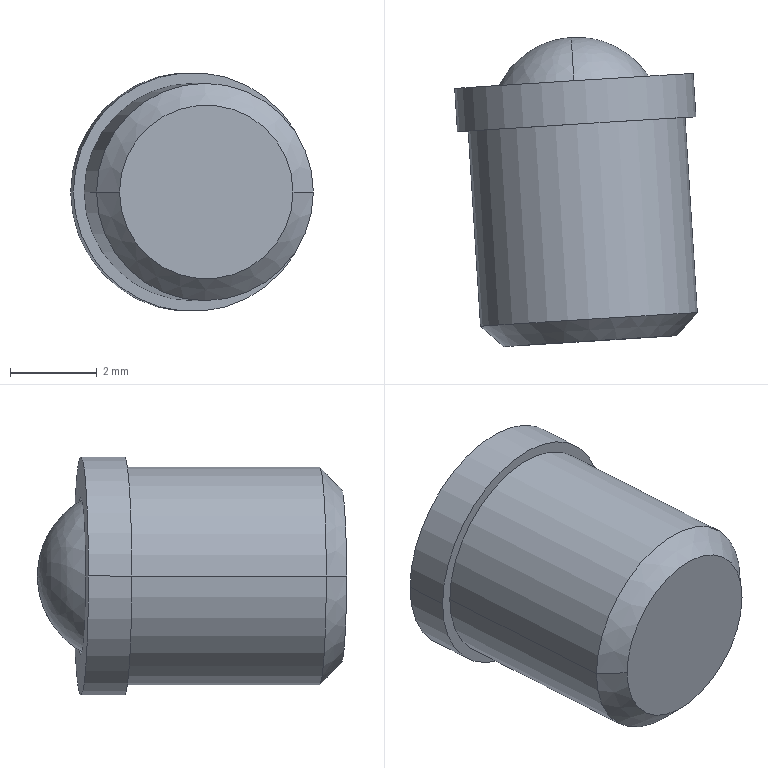Part | SolidWorks | features BaseBody 1 | 1 solid | 16 faces | box 5.585 x 7.116 x 5.5 mm | volume 124.528 mm3 | cylinder 8 | plane 4 | spline 2 | cone 2 | commonest cylinder face diameters 3.6 x2 4 x2 5 x2 5.5 x2
STEP:
#1=CARTESIAN_POINT('',(586.994,-147.553,58.889));
#2=VERTEX_POINT('',#1);
#3=CARTESIAN_POINT('',(588.99,-147.428,60.889));
#4=VERTEX_POINT('',#3);
#5=CARTESIAN_POINT('',(588.99,-147.428,58.889));
#6=DIRECTION('',(-0.06274,0.998,0.000000003));
#7=DIRECTION('',(-0.998,-0.06274,0.));
#8=AXIS2_PLACEMENT_3D('',#5,#6,#7);
#9=CIRCLE('',#8,2.);
#10=EDGE_CURVE('',#2,#4,#9,.T.);
#11=ORIENTED_EDGE('',*,*,#10,.T.);
#12=CARTESIAN_POINT('',(588.865,-145.432,58.889));
#13=VERTEX_POINT('',#12);
#14=CARTESIAN_POINT('',(588.99,-147.428,58.889));
#15=DIRECTION('',(-0.998,-0.06274,0.));
#16=DIRECTION('',(0.06274,-0.998,-0.000000003));
#17=AXIS2_PLACEMENT_3D('',#14,#15,#16);
#18=CIRCLE('',#17,2.);
#19=EDGE_CURVE('',#4,#13,#18,.T.);
#20=ORIENTED_EDGE('',*,*,#19,.T.);
#21=CARTESIAN_POINT('',(588.99,-147.428,56.889));
#22=VERTEX_POINT('',#21);
#23=CARTESIAN_POINT('',(588.99,-147.428,58.889));
#24=DIRECTION('',(0.998,0.06274,0.));
#25=DIRECTION('',(0.06274,-0.998,-0.000000003));
#26=AXIS2_PLACEMENT_3D('',#23,#24,#25);
#27=CIRCLE('',#26,2.);
#28=EDGE_CURVE('',#22,#13,#27,.T.);
#29=ORIENTED_EDGE('',*,*,#28,.F.);
#30=CARTESIAN_POINT('',(588.99,-147.428,58.889));
#31=DIRECTION('',(-0.06274,0.998,0.000000003));
#32=DIRECTION('',(-0.998,-0.06274,0.));
#33=AXIS2_PLACEMENT_3D('',#30,#31,#32);
#34=CIRCLE('',#33,2.);
#35=EDGE_CURVE('',#22,#2,#34,.T.);
#36=ORIENTED_EDGE('',*,*,#35,.T.);
#37=EDGE_LOOP('',(#11,#20,#29,#36));
#38=FACE_OUTER_BOUND('',#37,.T.);
#39=CARTESIAN_POINT('',(588.99,-147.428,60.889));
#40=CARTESIAN_POINT('',(584.998,-147.679,60.889));
#41=CARTESIAN_POINT('',(584.998,-147.679,56.889));
#42=CARTESIAN_POINT('',(588.99,-147.428,56.889));
#43=CARTESIAN_POINT('',(588.917,-146.258,60.889));
#44=CARTESIAN_POINT('',(584.925,-146.509,60.889));
#45=CARTESIAN_POINT('',(584.925,-146.509,56.889));
#46=CARTESIAN_POINT('',(588.917,-146.258,56.889));
#47=CARTESIAN_POINT('',(588.865,-145.432,60.06));
#48=CARTESIAN_POINT('',(586.526,-145.579,60.06));
#49=CARTESIAN_POINT('',(586.526,-145.579,57.717));
#50=CARTESIAN_POINT('',(588.865,-145.432,57.717));
#51=CARTESIAN_POINT('',(588.865,-145.432,58.889));
#52=CARTESIAN_POINT('',(588.865,-145.432,58.889));
#53=CARTESIAN_POINT('',(588.865,-145.432,58.889));
#54=CARTESIAN_POINT('',(588.865,-145.432,58.889));
#55=(BOUNDED_SURFACE()B_SPLINE_SURFACE(3,3,((#39,#40,#41,#42),(#43,#44,#45,#46),(#47,#48,#49,#50),(#51,#52,#53,#54)),.UNSPECIFIED.,.F.,.F.,.F.)B_SPLINE_SURFACE_WITH_KNOTS((4,4),(4,4),(0.,1.),(0.,1.),.UNSPECIFIED.)GEOMETRIC_REPRESENTATION_ITEM()RATIONAL_B_SPLINE_SURFACE(((1.,0.3333,0.3333,1.),(0.8047,0.2682,0.2682,0.8047),(0.8047,0.2682,0.2682,0.8047),(1.,0.3333,0.3333,1.)))REPRESENTATION_ITEM('')SURFACE());
#56=ADVANCED_FACE('',(#38),#55,.T.);
#57=CARTESIAN_POINT('',(586.778,-152.076,58.889));
#58=VERTEX_POINT('',#57);
#59=CARTESIAN_POINT('',(591.768,-151.762,58.889));
#60=VERTEX_POINT('',#59);
#61=CARTESIAN_POINT('',(589.273,-151.919,58.889));
#62=DIRECTION('',(-0.06274,0.998,0.000000003));
#63=DIRECTION('',(-0.998,-0.06274,0.));
#64=AXIS2_PLACEMENT_3D('',#61,#62,#63);
#65=CIRCLE('',#64,2.5);
#66=EDGE_CURVE('',#58,#60,#65,.T.);
#67=ORIENTED_EDGE('',*,*,#66,.T.);
#68=CARTESIAN_POINT('',(591.485,-147.271,58.889));
#69=VERTEX_POINT('',#68);
#70=CARTESIAN_POINT('',(591.338,-144.925,58.889));
#71=DIRECTION('',(-0.06274,0.998,0.000000003));
#72=VECTOR('',#71,1000.);
#73=LINE('',#70,#72);
#74=EDGE_CURVE('',#60,#69,#73,.T.);
#75=ORIENTED_EDGE('',*,*,#74,.T.);
#76=CARTESIAN_POINT('',(586.495,-147.584,58.889));
#77=VERTEX_POINT('',#76);
#78=CARTESIAN_POINT('',(588.99,-147.428,58.889));
#79=DIRECTION('',(0.06274,-0.998,-0.000000003));
#80=DIRECTION('',(-0.998,-0.06274,0.));
#81=AXIS2_PLACEMENT_3D('',#78,#79,#80);
#82=CIRCLE('',#81,2.5);
#83=EDGE_CURVE('',#69,#77,#82,.T.);
#84=ORIENTED_EDGE('',*,*,#83,.T.);
#85=CARTESIAN_POINT('',(586.348,-145.239,58.889));
#86=DIRECTION('',(-0.06274,0.998,0.000000003));
#87=VECTOR('',#86,1000.);
#88=LINE('',#85,#87);
#89=EDGE_CURVE('',#58,#77,#88,.T.);
#90=ORIENTED_EDGE('',*,*,#89,.F.);
#91=EDGE_LOOP('',(#67,#75,#84,#90));
#92=FACE_OUTER_BOUND('',#91,.T.);
#93=CARTESIAN_POINT('',(588.843,-145.082,58.889));
#94=DIRECTION('',(-0.06274,0.998,0.000000003));
#95=DIRECTION('',(-0.998,-0.06274,0.));
#96=AXIS2_PLACEMENT_3D('',#93,#94,#95);
#97=CYLINDRICAL_SURFACE('',#96,2.5);
#98=ADVANCED_FACE('',(#92),#97,.T.);
#99=CARTESIAN_POINT('',(587.308,-152.543,58.889));
#100=VERTEX_POINT('',#99);
#101=CARTESIAN_POINT('',(591.3,-152.292,58.889));
#102=VERTEX_POINT('',#101);
#103=CARTESIAN_POINT('',(589.304,-152.418,58.889));
#104=DIRECTION('',(-0.06274,0.998,0.000000003));
#105=DIRECTION('',(-0.998,-0.06274,0.));
#106=AXIS2_PLACEMENT_3D('',#103,#104,#105);
#107=CIRCLE('',#106,2.);
#108=EDGE_CURVE('',#100,#102,#107,.T.);
#109=ORIENTED_EDGE('',*,*,#108,.T.);
#110=CARTESIAN_POINT('',(591.768,-151.762,58.889));
#111=DIRECTION('',(0.6614,0.7501,0.000000002));
#112=VECTOR('',#111,1000.);
#113=LINE('',#110,#112);
#114=EDGE_CURVE('',#102,#60,#113,.T.);
#115=ORIENTED_EDGE('',*,*,#114,.T.);
#116=ORIENTED_EDGE('',*,*,#66,.F.);
#117=CARTESIAN_POINT('',(586.778,-152.076,58.889));
#118=DIRECTION('',(-0.7501,0.6614,0.000000002));
#119=VECTOR('',#118,1000.);
#120=LINE('',#117,#119);
#121=EDGE_CURVE('',#100,#58,#120,.T.);
#122=ORIENTED_EDGE('',*,*,#121,.F.);
#123=EDGE_LOOP('',(#109,#115,#116,#122));
#124=FACE_OUTER_BOUND('',#123,.T.);
#125=CARTESIAN_POINT('',(589.273,-151.919,58.889));
#126=DIRECTION('',(-0.06274,0.998,0.000000003));
#127=DIRECTION('',(-0.998,-0.06274,0.));
#128=AXIS2_PLACEMENT_3D('',#125,#126,#127);
#129=CONICAL_SURFACE('',#128,2.5,0.7854);
#130=ADVANCED_FACE('',(#124),#129,.T.);
#131=CARTESIAN_POINT('',(591.735,-147.255,58.889));
#132=VERTEX_POINT('',#131);
#133=CARTESIAN_POINT('',(586.246,-147.6,58.889));
#134=VERTEX_POINT('',#133);
#135=CARTESIAN_POINT('',(588.99,-147.428,58.889));
#136=DIRECTION('',(0.06274,-0.998,-0.000000003));
#137=DIRECTION('',(-0.998,-0.06274,0.));
#138=AXIS2_PLACEMENT_3D('',#135,#136,#137);
#139=CIRCLE('',#138,2.75);
#140=EDGE_CURVE('',#132,#134,#139,.T.);
#141=ORIENTED_EDGE('',*,*,#140,.F.);
#142=CARTESIAN_POINT('',(591.672,-146.257,58.889));
#143=VERTEX_POINT('',#142);
#144=CARTESIAN_POINT('',(591.587,-144.91,58.889));
#145=DIRECTION('',(-0.06274,0.998,0.000000003));
#146=VECTOR('',#145,1000.);
#147=LINE('',#144,#146);
#148=EDGE_CURVE('',#132,#143,#147,.T.);
#149=ORIENTED_EDGE('',*,*,#148,.T.);
#150=CARTESIAN_POINT('',(586.183,-146.602,58.889));
#151=VERTEX_POINT('',#150);
#152=CARTESIAN_POINT('',(588.928,-146.43,58.889));
#153=DIRECTION('',(0.06274,-0.998,-0.000000003));
#154=DIRECTION('',(-0.998,-0.06274,0.));
#155=AXIS2_PLACEMENT_3D('',#152,#153,#154);
#156=CIRCLE('',#155,2.75);
#157=EDGE_CURVE('',#143,#151,#156,.T.);
#158=ORIENTED_EDGE('',*,*,#157,.T.);
#159=CARTESIAN_POINT('',(586.098,-145.255,58.889));
#160=DIRECTION('',(-0.06274,0.998,0.000000003));
#161=VECTOR('',#160,1000.);
#162=LINE('',#159,#161);
#163=EDGE_CURVE('',#134,#151,#162,.T.);
#164=ORIENTED_EDGE('',*,*,#163,.F.);
#165=EDGE_LOOP('',(#141,#149,#158,#164));
#166=FACE_OUTER_BOUND('',#165,.T.);
#167=CARTESIAN_POINT('',(588.843,-145.082,58.889));
#168=DIRECTION('',(-0.06274,0.998,0.000000003));
#169=DIRECTION('',(-0.998,-0.06274,0.));
#170=AXIS2_PLACEMENT_3D('',#167,#168,#169);
#171=CYLINDRICAL_SURFACE('',#170,2.75);
#172=ADVANCED_FACE('',(#166),#171,.T.);
#173=CARTESIAN_POINT('',(590.73,-146.416,58.889));
#174=VERTEX_POINT('',#173);
#175=CARTESIAN_POINT('',(587.137,-146.642,58.889));
#176=VERTEX_POINT('',#175);
#177=CARTESIAN_POINT('',(588.934,-146.529,58.889));
#178=DIRECTION('',(-0.06274,0.998,0.000000003));
#179=DIRECTION('',(-0.998,-0.06274,0.));
#180=AXIS2_PLACEMENT_3D('',#177,#178,#179);
#181=CIRCLE('',#180,1.8);
#182=EDGE_CURVE('',#174,#176,#181,.T.);
#183=ORIENTED_EDGE('',*,*,#182,.F.);
#184=CARTESIAN_POINT('',(590.724,-146.317,58.889));
#185=VERTEX_POINT('',#184);
#186=CARTESIAN_POINT('',(590.639,-144.969,58.889));
#187=DIRECTION('',(-0.06274,0.998,0.000000003));
#188=VECTOR('',#187,1000.);
#189=LINE('',#186,#188);
#190=EDGE_CURVE('',#174,#185,#189,.T.);
#191=ORIENTED_EDGE('',*,*,#190,.T.);
#192=CARTESIAN_POINT('',(587.131,-146.543,58.889));
#193=VERTEX_POINT('',#192);
#194=CARTESIAN_POINT('',(588.928,-146.43,58.889));
#195=DIRECTION('',(-0.06274,0.998,0.000000003));
#196=DIRECTION('',(-0.998,-0.06274,0.));
#197=AXIS2_PLACEMENT_3D('',#194,#195,#196);
#198=CIRCLE('',#197,1.8);
#199=EDGE_CURVE('',#185,#193,#198,.T.);
#200=ORIENTED_EDGE('',*,*,#199,.T.);
#201=CARTESIAN_POINT('',(587.046,-145.195,58.889));
#202=DIRECTION('',(-0.06274,0.998,0.000000003));
#203=VECTOR('',#202,1000.);
#204=LINE('',#201,#203);
#205=EDGE_CURVE('',#176,#193,#204,.T.);
#206=ORIENTED_EDGE('',*,*,#205,.F.);
#207=EDGE_LOOP('',(#183,#191,#200,#206));
#208=FACE_OUTER_BOUND('',#207,.T.);
#209=CARTESIAN_POINT('',(588.843,-145.082,58.889));
#210=DIRECTION('',(-0.06274,0.998,0.000000003));
#211=DIRECTION('',(-0.998,-0.06274,0.));
#212=AXIS2_PLACEMENT_3D('',#209,#210,#211);
#213=CYLINDRICAL_SURFACE('',#212,1.8);
#214=ADVANCED_FACE('',(#208),#213,.F.);
#215=CARTESIAN_POINT('',(590.986,-147.302,58.889));
#216=VERTEX_POINT('',#215);
#217=CARTESIAN_POINT('',(588.99,-147.428,58.889));
#218=DIRECTION('',(-0.06274,0.998,0.000000003));
#219=DIRECTION('',(-0.998,-0.06274,0.));
#220=AXIS2_PLACEMENT_3D('',#217,#218,#219);
#221=CIRCLE('',#220,2.);
#222=EDGE_CURVE('',#216,#22,#221,.T.);
#223=ORIENTED_EDGE('',*,*,#222,.F.);
#224=CARTESIAN_POINT('',(590.93,-146.404,58.889));
#225=VERTEX_POINT('',#224);
#226=CARTESIAN_POINT('',(590.839,-144.957,58.889));
#227=DIRECTION('',(-0.06274,0.998,0.000000003));
#228=VECTOR('',#227,1000.);
#229=LINE('',#226,#228);
#230=EDGE_CURVE('',#216,#225,#229,.T.);
#231=ORIENTED_EDGE('',*,*,#230,.T.);
#232=CARTESIAN_POINT('',(586.938,-146.655,58.889));
#233=VERTEX_POINT('',#232);
#234=CARTESIAN_POINT('',(588.934,-146.529,58.889));
#235=DIRECTION('',(0.06274,-0.998,-0.000000003));
#236=DIRECTION('',(-0.998,-0.06274,0.));
#237=AXIS2_PLACEMENT_3D('',#234,#235,#236);
#238=CIRCLE('',#237,2.);
#239=EDGE_CURVE('',#233,#225,#238,.T.);
#240=ORIENTED_EDGE('',*,*,#239,.F.);
#241=CARTESIAN_POINT('',(586.847,-145.208,58.889));
#242=DIRECTION('',(-0.06274,0.998,0.000000003));
#243=VECTOR('',#242,1000.);
#244=LINE('',#241,#243);
#245=EDGE_CURVE('',#2,#233,#244,.T.);
#246=ORIENTED_EDGE('',*,*,#245,.F.);
#247=ORIENTED_EDGE('',*,*,#35,.F.);
#248=EDGE_LOOP('',(#223,#231,#240,#246,#247));
#249=FACE_OUTER_BOUND('',#248,.T.);
#250=CARTESIAN_POINT('',(588.843,-145.082,58.889));
#251=DIRECTION('',(-0.06274,0.998,0.000000003));
#252=DIRECTION('',(-0.998,-0.06274,0.));
#253=AXIS2_PLACEMENT_3D('',#250,#251,#252);
#254=CYLINDRICAL_SURFACE('',#253,2.);
#255=ADVANCED_FACE('',(#249),#254,.F.);
#256=ORIENTED_EDGE('',*,*,#74,.F.);
#257=CARTESIAN_POINT('',(589.273,-151.919,58.889));
#258=DIRECTION('',(-0.06274,0.998,0.000000003));
#259=DIRECTION('',(-0.998,-0.06274,0.));
#260=AXIS2_PLACEMENT_3D('',#257,#258,#259);
#261=CIRCLE('',#260,2.5);
#262=EDGE_CURVE('',#60,#58,#261,.T.);
#263=ORIENTED_EDGE('',*,*,#262,.T.);
#264=ORIENTED_EDGE('',*,*,#89,.T.);
#265=CARTESIAN_POINT('',(588.99,-147.428,58.889));
#266=DIRECTION('',(0.06274,-0.998,-0.000000003));
#267=DIRECTION('',(-0.998,-0.06274,0.));
#268=AXIS2_PLACEMENT_3D('',#265,#266,#267);
#269=CIRCLE('',#268,2.5);
#270=EDGE_CURVE('',#77,#69,#269,.T.);
#271=ORIENTED_EDGE('',*,*,#270,.T.);
#272=EDGE_LOOP('',(#256,#263,#264,#271));
#273=FACE_OUTER_BOUND('',#272,.T.);
#274=CARTESIAN_POINT('',(588.843,-145.082,58.889));
#275=DIRECTION('',(-0.06274,0.998,0.000000003));
#276=DIRECTION('',(-0.998,-0.06274,0.));
#277=AXIS2_PLACEMENT_3D('',#274,#275,#276);
#278=CYLINDRICAL_SURFACE('',#277,2.5);
#279=ADVANCED_FACE('',(#273),#278,.T.);
#280=ORIENTED_EDGE('',*,*,#270,.F.);
#281=ORIENTED_EDGE('',*,*,#83,.F.);
#282=EDGE_LOOP('',(#280,#281));
#283=FACE_BOUND('',#282,.T.);
#284=CARTESIAN_POINT('',(588.99,-147.428,58.889));
#285=DIRECTION('',(0.06274,-0.998,-0.000000003));
#286=DIRECTION('',(-0.998,-0.06274,0.));
#287=AXIS2_PLACEMENT_3D('',#284,#285,#286);
#288=CIRCLE('',#287,2.75);
#289=EDGE_CURVE('',#134,#132,#288,.T.);
#290=ORIENTED_EDGE('',*,*,#289,.T.);
#291=ORIENTED_EDGE('',*,*,#140,.T.);
#292=EDGE_LOOP('',(#290,#291));
#293=FACE_OUTER_BOUND('',#292,.T.);
#294=CARTESIAN_POINT('',(588.99,-147.428,58.889));
#295=DIRECTION('',(0.06274,-0.998,-0.000000003));
#296=DIRECTION('',(0.998,0.06274,0.));
#297=AXIS2_PLACEMENT_3D('',#294,#295,#296);
#298=PLANE('',#297);
#299=ADVANCED_FACE('',(#283,#293),#298,.T.);
#300=ORIENTED_EDGE('',*,*,#114,.F.);
#301=CARTESIAN_POINT('',(589.304,-152.418,58.889));
#302=DIRECTION('',(-0.06274,0.998,0.000000003));
#303=DIRECTION('',(-0.998,-0.06274,0.));
#304=AXIS2_PLACEMENT_3D('',#301,#302,#303);
#305=CIRCLE('',#304,2.);
#306=EDGE_CURVE('',#102,#100,#305,.T.);
#307=ORIENTED_EDGE('',*,*,#306,.T.);
#308=ORIENTED_EDGE('',*,*,#121,.T.);
#309=ORIENTED_EDGE('',*,*,#262,.F.);
#310=EDGE_LOOP('',(#300,#307,#308,#309));
#311=FACE_OUTER_BOUND('',#310,.T.);
#312=CARTESIAN_POINT('',(589.273,-151.919,58.889));
#313=DIRECTION('',(-0.06274,0.998,0.000000003));
#314=DIRECTION('',(-0.998,-0.06274,0.));
#315=AXIS2_PLACEMENT_3D('',#312,#313,#314);
#316=CONICAL_SURFACE('',#315,2.5,0.7854);
#317=ADVANCED_FACE('',(#311),#316,.T.);
#318=ORIENTED_EDGE('',*,*,#148,.F.);
#319=ORIENTED_EDGE('',*,*,#289,.F.);
#320=ORIENTED_EDGE('',*,*,#163,.T.);
#321=CARTESIAN_POINT('',(588.928,-146.43,58.889));
#322=DIRECTION('',(0.06274,-0.998,-0.000000003));
#323=DIRECTION('',(-0.998,-0.06274,0.));
#324=AXIS2_PLACEMENT_3D('',#321,#322,#323);
#325=CIRCLE('',#324,2.75);
#326=EDGE_CURVE('',#151,#143,#325,.T.);
#327=ORIENTED_EDGE('',*,*,#326,.T.);
#328=EDGE_LOOP('',(#318,#319,#320,#327));
#329=FACE_OUTER_BOUND('',#328,.T.);
#330=CARTESIAN_POINT('',(588.843,-145.082,58.889));
#331=DIRECTION('',(-0.06274,0.998,0.000000003));
#332=DIRECTION('',(-0.998,-0.06274,0.));
#333=AXIS2_PLACEMENT_3D('',#330,#331,#332);
#334=CYLINDRICAL_SURFACE('',#333,2.75);
#335=ADVANCED_FACE('',(#329),#334,.T.);
#336=ORIENTED_EDGE('',*,*,#108,.F.);
#337=ORIENTED_EDGE('',*,*,#306,.F.);
#338=EDGE_LOOP('',(#336,#337));
#339=FACE_OUTER_BOUND('',#338,.T.);
#340=CARTESIAN_POINT('',(589.304,-152.418,58.889));
#341=DIRECTION('',(0.06274,-0.998,-0.000000003));
#342=DIRECTION('',(0.998,0.06274,0.));
#343=AXIS2_PLACEMENT_3D('',#340,#341,#342);
#344=PLANE('',#343);
#345=ADVANCED_FACE('',(#339),#344,.T.);
#346=CARTESIAN_POINT('',(588.928,-146.43,58.889));
#347=DIRECTION('',(-0.06274,0.998,0.000000003));
#348=DIRECTION('',(-0.998,-0.06274,0.));
#349=AXIS2_PLACEMENT_3D('',#346,#347,#348);
#350=CIRCLE('',#349,1.8);
#351=EDGE_CURVE('',#193,#185,#350,.T.);
#352=ORIENTED_EDGE('',*,*,#351,.F.);
#353=ORIENTED_EDGE('',*,*,#199,.F.);
#354=EDGE_LOOP('',(#352,#353));
#355=FACE_BOUND('',#354,.T.);
#356=ORIENTED_EDGE('',*,*,#326,.F.);
#357=ORIENTED_EDGE('',*,*,#157,.F.);
#358=EDGE_LOOP('',(#356,#357));
#359=FACE_OUTER_BOUND('',#358,.T.);
#360=CARTESIAN_POINT('',(588.928,-146.43,58.889));
#361=DIRECTION('',(0.06274,-0.998,-0.000000003));
#362=DIRECTION('',(0.998,0.06274,0.));
#363=AXIS2_PLACEMENT_3D('',#360,#361,#362);
#364=PLANE('',#363);
#365=ADVANCED_FACE('',(#355,#359),#364,.F.);
#366=ORIENTED_EDGE('',*,*,#190,.F.);
#367=CARTESIAN_POINT('',(588.934,-146.529,58.889));
#368=DIRECTION('',(-0.06274,0.998,0.000000003));
#369=DIRECTION('',(-0.998,-0.06274,0.));
#370=AXIS2_PLACEMENT_3D('',#367,#368,#369);
#371=CIRCLE('',#370,1.8);
#372=EDGE_CURVE('',#176,#174,#371,.T.);
#373=ORIENTED_EDGE('',*,*,#372,.F.);
#374=ORIENTED_EDGE('',*,*,#205,.T.);
#375=ORIENTED_EDGE('',*,*,#351,.T.);
#376=EDGE_LOOP('',(#366,#373,#374,#375));
#377=FACE_OUTER_BOUND('',#376,.T.);
#378=CARTESIAN_POINT('',(588.843,-145.082,58.889));
#379=DIRECTION('',(-0.06274,0.998,0.000000003));
#380=DIRECTION('',(-0.998,-0.06274,0.));
#381=AXIS2_PLACEMENT_3D('',#378,#379,#380);
#382=CYLINDRICAL_SURFACE('',#381,1.8);
#383=ADVANCED_FACE('',(#377),#382,.F.);
#384=ORIENTED_EDGE('',*,*,#372,.T.);
#385=ORIENTED_EDGE('',*,*,#182,.T.);
#386=EDGE_LOOP('',(#384,#385));
#387=FACE_BOUND('',#386,.T.);
#388=ORIENTED_EDGE('',*,*,#239,.T.);
#389=CARTESIAN_POINT('',(588.934,-146.529,58.889));
#390=DIRECTION('',(0.06274,-0.998,-0.000000003));
#391=DIRECTION('',(-0.998,-0.06274,0.));
#392=AXIS2_PLACEMENT_3D('',#389,#390,#391);
#393=CIRCLE('',#392,2.);
#394=EDGE_CURVE('',#225,#233,#393,.T.);
#395=ORIENTED_EDGE('',*,*,#394,.T.);
#396=EDGE_LOOP('',(#388,#395));
#397=FACE_OUTER_BOUND('',#396,.T.);
#398=CARTESIAN_POINT('',(588.934,-146.529,58.889));
#399=DIRECTION('',(0.06274,-0.998,-0.000000003));
#400=DIRECTION('',(0.998,0.06274,0.));
#401=AXIS2_PLACEMENT_3D('',#398,#399,#400);
#402=PLANE('',#401);
#403=ADVANCED_FACE('',(#387,#397),#402,.T.);
#404=ORIENTED_EDGE('',*,*,#230,.F.);
#405=CARTESIAN_POINT('',(588.99,-147.428,58.889));
#406=DIRECTION('',(-0.06274,0.998,0.000000003));
#407=DIRECTION('',(-0.998,-0.06274,0.));
#408=AXIS2_PLACEMENT_3D('',#405,#406,#407);
#409=CIRCLE('',#408,2.);
#410=EDGE_CURVE('',#4,#216,#409,.T.);
#411=ORIENTED_EDGE('',*,*,#410,.F.);
#412=ORIENTED_EDGE('',*,*,#10,.F.);
#413=ORIENTED_EDGE('',*,*,#245,.T.);
#414=ORIENTED_EDGE('',*,*,#394,.F.);
#415=EDGE_LOOP('',(#404,#411,#412,#413,#414));
#416=FACE_OUTER_BOUND('',#415,.T.);
#417=CARTESIAN_POINT('',(588.843,-145.082,58.889));
#418=DIRECTION('',(-0.06274,0.998,0.000000003));
#419=DIRECTION('',(-0.998,-0.06274,0.));
#420=AXIS2_PLACEMENT_3D('',#417,#418,#419);
#421=CYLINDRICAL_SURFACE('',#420,2.);
#422=ADVANCED_FACE('',(#416),#421,.F.);
#423=ORIENTED_EDGE('',*,*,#19,.F.);
#424=ORIENTED_EDGE('',*,*,#410,.T.);
#425=ORIENTED_EDGE('',*,*,#222,.T.);
#426=ORIENTED_EDGE('',*,*,#28,.T.);
#427=EDGE_LOOP('',(#423,#424,#425,#426));
#428=FACE_OUTER_BOUND('',#427,.T.);
#429=CARTESIAN_POINT('',(588.99,-147.428,56.889));
#430=CARTESIAN_POINT('',(592.982,-147.177,56.889));
#431=CARTESIAN_POINT('',(592.982,-147.177,60.889));
#432=CARTESIAN_POINT('',(588.99,-147.428,60.889));
#433=CARTESIAN_POINT('',(588.917,-146.258,56.889));
#434=CARTESIAN_POINT('',(592.909,-146.007,56.889));
#435=CARTESIAN_POINT('',(592.909,-146.007,60.889));
#436=CARTESIAN_POINT('',(588.917,-146.258,60.889));
#437=CARTESIAN_POINT('',(588.865,-145.432,57.717));
#438=CARTESIAN_POINT('',(591.203,-145.285,57.717));
#439=CARTESIAN_POINT('',(591.203,-145.285,60.06));
#440=CARTESIAN_POINT('',(588.865,-145.432,60.06));
#441=CARTESIAN_POINT('',(588.865,-145.432,58.889));
#442=CARTESIAN_POINT('',(588.865,-145.432,58.889));
#443=CARTESIAN_POINT('',(588.865,-145.432,58.889));
#444=CARTESIAN_POINT('',(588.865,-145.432,58.889));
#445=(BOUNDED_SURFACE()B_SPLINE_SURFACE(3,3,((#429,#430,#431,#432),(#433,#434,#435,#436),(#437,#438,#439,#440),(#441,#442,#443,#444)),.UNSPECIFIED.,.F.,.F.,.F.)B_SPLINE_SURFACE_WITH_KNOTS((4,4),(4,4),(0.,1.),(0.,1.),.UNSPECIFIED.)GEOMETRIC_REPRESENTATION_ITEM()RATIONAL_B_SPLINE_SURFACE(((1.,0.3333,0.3333,1.),(0.8047,0.2682,0.2682,0.8047),(0.8047,0.2682,0.2682,0.8047),(1.,0.3333,0.3333,1.)))REPRESENTATION_ITEM('')SURFACE());
#446=ADVANCED_FACE('',(#428),#445,.T.);
#447=CLOSED_SHELL('',(#56,#98,#130,#172,#214,#255,#279,#299,#317,#335,#345,#365,#383,#403,#422,#446));
#448=MANIFOLD_SOLID_BREP('',#447);
#449=CARTESIAN_POINT('',(0.,0.,0.));
#450=DIRECTION('',(0.,0.,1.));
#451=DIRECTION('',(1.,0.,0.));
#452=AXIS2_PLACEMENT_3D('',#449,#450,#451);
#453=(LENGTH_UNIT()NAMED_UNIT(*)SI_UNIT(.MILLI.,.METRE.));
#454=UNCERTAINTY_MEASURE_WITH_UNIT(LENGTH_MEASURE(0.00001),#453,'','');
#455=(NAMED_UNIT(*)PLANE_ANGLE_UNIT()SI_UNIT($,.RADIAN.));
#456=(NAMED_UNIT(*)SI_UNIT($,.STERADIAN.)SOLID_ANGLE_UNIT());
#457=(GEOMETRIC_REPRESENTATION_CONTEXT(3)GLOBAL_UNCERTAINTY_ASSIGNED_CONTEXT((#454))GLOBAL_UNIT_ASSIGNED_CONTEXT((#453,#455,#456))REPRESENTATION_CONTEXT('',''));
#458=ADVANCED_BREP_SHAPE_REPRESENTATION('',(#448,#452),#457);